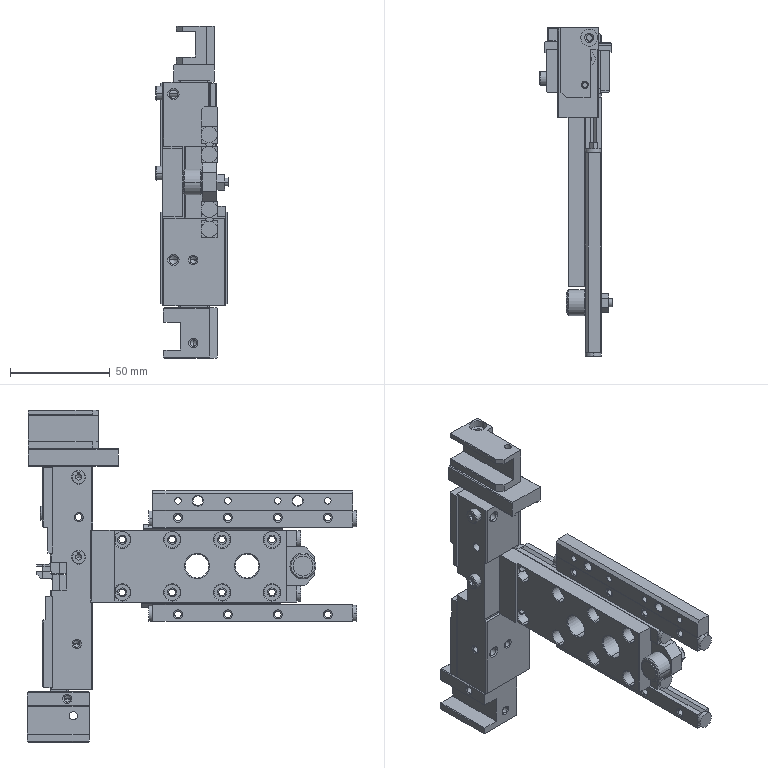Part | NX | 26 solids | 1135 faces | box 36.3 x 164.9 x 166.238 mm | volume 171770 mm3 | plane 563 | cylinder 335 | cone 237 | commonest cylinder face diameters 3.3 x74 6 x44 8 x40 4.5 x33 5 x32 3 x22